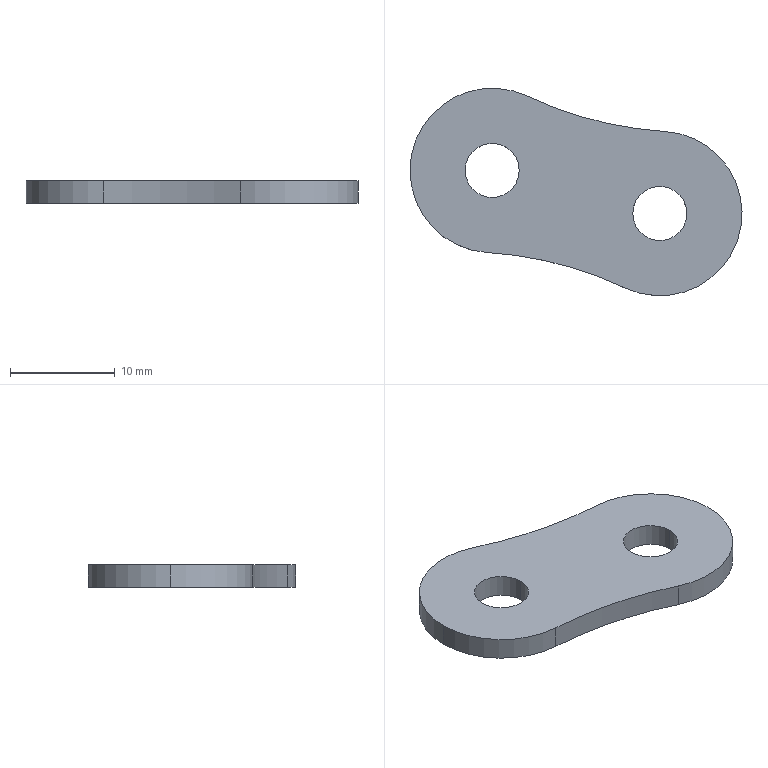Part | SolidWorks | features Boss 2, DeleteBody 1, Extrusion 1, Scale 1 | 1 solid | 11 faces | box 31.676 x 19.79 x 2.171 mm | volume 856.64 mm3 | cylinder 9 | plane 2 | commonest cylinder face diameters 5.161 x4 15.684 x2 71.994 x2 15.685 x1
STEP:
#1=CARTESIAN_POINT('',(21.666,-4.106,9.519));
#2=VERTEX_POINT('',#1);
#3=CARTESIAN_POINT('',(26.827,-4.106,9.519));
#4=VERTEX_POINT('',#3);
#5=CARTESIAN_POINT('',(24.246,-4.106,9.519));
#6=DIRECTION('',(0.,0.,1.));
#7=DIRECTION('',(1.,0.,0.));
#8=AXIS2_PLACEMENT_3D('',#5,#6,#7);
#9=CIRCLE('',#8,2.581);
#10=EDGE_CURVE('',#2,#4,#9,.T.);
#11=ORIENTED_EDGE('',*,*,#10,.T.);
#12=CARTESIAN_POINT('',(26.827,-4.106,7.348));
#13=VERTEX_POINT('',#12);
#14=CARTESIAN_POINT('',(26.827,-4.106,9.519));
#15=DIRECTION('',(0.,0.,-1.));
#16=VECTOR('',#15,1000.);
#17=LINE('',#14,#16);
#18=EDGE_CURVE('',#4,#13,#17,.T.);
#19=ORIENTED_EDGE('',*,*,#18,.T.);
#20=CARTESIAN_POINT('',(21.666,-4.106,7.348));
#21=VERTEX_POINT('',#20);
#22=CARTESIAN_POINT('',(24.246,-4.106,7.348));
#23=DIRECTION('',(0.,0.,1.));
#24=DIRECTION('',(1.,0.,0.));
#25=AXIS2_PLACEMENT_3D('',#22,#23,#24);
#26=CIRCLE('',#25,2.581);
#27=EDGE_CURVE('',#21,#13,#26,.T.);
#28=ORIENTED_EDGE('',*,*,#27,.F.);
#29=CARTESIAN_POINT('',(21.666,-4.106,9.519));
#30=DIRECTION('',(0.,0.,-1.));
#31=VECTOR('',#30,1000.);
#32=LINE('',#29,#31);
#33=EDGE_CURVE('',#2,#21,#32,.T.);
#34=ORIENTED_EDGE('',*,*,#33,.F.);
#35=EDGE_LOOP('',(#11,#19,#28,#34));
#36=FACE_OUTER_BOUND('',#35,.T.);
#37=CARTESIAN_POINT('',(24.246,-4.106,9.519));
#38=DIRECTION('',(0.,0.,-1.));
#39=DIRECTION('',(-1.,0.,0.));
#40=AXIS2_PLACEMENT_3D('',#37,#38,#39);
#41=CYLINDRICAL_SURFACE('',#40,2.581);
#42=ADVANCED_FACE('',(#36),#41,.F.);
#43=CARTESIAN_POINT('',(5.675,0.,9.519));
#44=VERTEX_POINT('',#43);
#45=CARTESIAN_POINT('',(10.836,0.,9.519));
#46=VERTEX_POINT('',#45);
#47=CARTESIAN_POINT('',(8.255,0.,9.519));
#48=DIRECTION('',(0.,0.,1.));
#49=DIRECTION('',(1.,0.,0.));
#50=AXIS2_PLACEMENT_3D('',#47,#48,#49);
#51=CIRCLE('',#50,2.58);
#52=EDGE_CURVE('',#44,#46,#51,.T.);
#53=ORIENTED_EDGE('',*,*,#52,.T.);
#54=CARTESIAN_POINT('',(10.836,0.,7.348));
#55=VERTEX_POINT('',#54);
#56=CARTESIAN_POINT('',(10.836,0.,9.519));
#57=DIRECTION('',(0.,0.,-1.));
#58=VECTOR('',#57,1000.);
#59=LINE('',#56,#58);
#60=EDGE_CURVE('',#46,#55,#59,.T.);
#61=ORIENTED_EDGE('',*,*,#60,.T.);
#62=CARTESIAN_POINT('',(5.675,0.,7.348));
#63=VERTEX_POINT('',#62);
#64=CARTESIAN_POINT('',(8.255,0.,7.348));
#65=DIRECTION('',(0.,0.,1.));
#66=DIRECTION('',(1.,0.,0.));
#67=AXIS2_PLACEMENT_3D('',#64,#65,#66);
#68=CIRCLE('',#67,2.58);
#69=EDGE_CURVE('',#63,#55,#68,.T.);
#70=ORIENTED_EDGE('',*,*,#69,.F.);
#71=CARTESIAN_POINT('',(5.675,0.,9.519));
#72=DIRECTION('',(0.,0.,-1.));
#73=VECTOR('',#72,1000.);
#74=LINE('',#71,#73);
#75=EDGE_CURVE('',#44,#63,#74,.T.);
#76=ORIENTED_EDGE('',*,*,#75,.F.);
#77=EDGE_LOOP('',(#53,#61,#70,#76));
#78=FACE_OUTER_BOUND('',#77,.T.);
#79=CARTESIAN_POINT('',(8.255,0.,9.519));
#80=DIRECTION('',(0.,0.,-1.));
#81=DIRECTION('',(-1.,0.,0.));
#82=AXIS2_PLACEMENT_3D('',#79,#80,#81);
#83=CYLINDRICAL_SURFACE('',#82,2.581);
#84=ADVANCED_FACE('',(#78),#83,.F.);
#85=CARTESIAN_POINT('',(0.4128,0.,9.519));
#86=VERTEX_POINT('',#85);
#87=CARTESIAN_POINT('',(7.77,-7.827,9.519));
#88=VERTEX_POINT('',#87);
#89=CARTESIAN_POINT('',(8.255,0.,9.519));
#90=DIRECTION('',(0.,0.,1.));
#91=DIRECTION('',(1.,0.,0.));
#92=AXIS2_PLACEMENT_3D('',#89,#90,#91);
#93=CIRCLE('',#92,7.842);
#94=EDGE_CURVE('',#86,#88,#93,.T.);
#95=ORIENTED_EDGE('',*,*,#94,.F.);
#96=CARTESIAN_POINT('',(0.4128,0.,7.348));
#97=VERTEX_POINT('',#96);
#98=CARTESIAN_POINT('',(0.4128,0.,9.519));
#99=DIRECTION('',(0.,0.,-1.));
#100=VECTOR('',#99,1000.);
#101=LINE('',#98,#100);
#102=EDGE_CURVE('',#86,#97,#101,.T.);
#103=ORIENTED_EDGE('',*,*,#102,.T.);
#104=CARTESIAN_POINT('',(7.77,-7.827,7.348));
#105=VERTEX_POINT('',#104);
#106=CARTESIAN_POINT('',(8.255,0.,7.348));
#107=DIRECTION('',(0.,0.,1.));
#108=DIRECTION('',(1.,0.,0.));
#109=AXIS2_PLACEMENT_3D('',#106,#107,#108);
#110=CIRCLE('',#109,7.842);
#111=EDGE_CURVE('',#97,#105,#110,.T.);
#112=ORIENTED_EDGE('',*,*,#111,.T.);
#113=CARTESIAN_POINT('',(7.77,-7.827,9.519));
#114=DIRECTION('',(0.,0.,-1.));
#115=VECTOR('',#114,1000.);
#116=LINE('',#113,#115);
#117=EDGE_CURVE('',#88,#105,#116,.T.);
#118=ORIENTED_EDGE('',*,*,#117,.F.);
#119=EDGE_LOOP('',(#95,#103,#112,#118));
#120=FACE_OUTER_BOUND('',#119,.T.);
#121=CARTESIAN_POINT('',(8.255,0.,9.519));
#122=DIRECTION('',(0.,0.,-1.));
#123=DIRECTION('',(-1.,0.,0.));
#124=AXIS2_PLACEMENT_3D('',#121,#122,#123);
#125=CYLINDRICAL_SURFACE('',#124,7.842);
#126=ADVANCED_FACE('',(#120),#125,.T.);
#127=ORIENTED_EDGE('',*,*,#52,.F.);
#128=CARTESIAN_POINT('',(8.255,0.,9.519));
#129=DIRECTION('',(0.,0.,1.));
#130=DIRECTION('',(1.,0.,0.));
#131=AXIS2_PLACEMENT_3D('',#128,#129,#130);
#132=CIRCLE('',#131,2.58);
#133=EDGE_CURVE('',#46,#44,#132,.T.);
#134=ORIENTED_EDGE('',*,*,#133,.F.);
#135=EDGE_LOOP('',(#127,#134));
#136=FACE_BOUND('',#135,.T.);
#137=CARTESIAN_POINT('',(24.731,3.721,9.519));
#138=VERTEX_POINT('',#137);
#139=CARTESIAN_POINT('',(11.601,7.093,9.519));
#140=VERTEX_POINT('',#139);
#141=CARTESIAN_POINT('',(26.958,39.65,9.519));
#142=DIRECTION('',(0.,0.,-1.));
#143=DIRECTION('',(1.,0.,0.));
#144=AXIS2_PLACEMENT_3D('',#141,#142,#143);
#145=CIRCLE('',#144,35.997);
#146=EDGE_CURVE('',#138,#140,#145,.T.);
#147=ORIENTED_EDGE('',*,*,#146,.T.);
#148=CARTESIAN_POINT('',(8.255,0.,9.519));
#149=DIRECTION('',(0.,0.,1.));
#150=DIRECTION('',(1.,0.,0.));
#151=AXIS2_PLACEMENT_3D('',#148,#149,#150);
#152=CIRCLE('',#151,7.842);
#153=EDGE_CURVE('',#140,#86,#152,.T.);
#154=ORIENTED_EDGE('',*,*,#153,.T.);
#155=ORIENTED_EDGE('',*,*,#94,.T.);
#156=CARTESIAN_POINT('',(20.901,-11.199,9.519));
#157=VERTEX_POINT('',#156);
#158=CARTESIAN_POINT('',(5.543,-43.756,9.519));
#159=DIRECTION('',(0.,0.,-1.));
#160=DIRECTION('',(-1.,0.,0.));
#161=AXIS2_PLACEMENT_3D('',#158,#159,#160);
#162=CIRCLE('',#161,35.997);
#163=EDGE_CURVE('',#88,#157,#162,.T.);
#164=ORIENTED_EDGE('',*,*,#163,.T.);
#165=CARTESIAN_POINT('',(24.246,-4.106,9.519));
#166=DIRECTION('',(0.,0.,1.));
#167=DIRECTION('',(1.,0.,0.));
#168=AXIS2_PLACEMENT_3D('',#165,#166,#167);
#169=CIRCLE('',#168,7.842);
#170=EDGE_CURVE('',#157,#138,#169,.T.);
#171=ORIENTED_EDGE('',*,*,#170,.T.);
#172=EDGE_LOOP('',(#147,#154,#155,#164,#171));
#173=FACE_OUTER_BOUND('',#172,.T.);
#174=ORIENTED_EDGE('',*,*,#10,.F.);
#175=CARTESIAN_POINT('',(24.246,-4.106,9.519));
#176=DIRECTION('',(0.,0.,1.));
#177=DIRECTION('',(1.,0.,0.));
#178=AXIS2_PLACEMENT_3D('',#175,#176,#177);
#179=CIRCLE('',#178,2.581);
#180=EDGE_CURVE('',#4,#2,#179,.T.);
#181=ORIENTED_EDGE('',*,*,#180,.F.);
#182=EDGE_LOOP('',(#174,#181));
#183=FACE_BOUND('',#182,.T.);
#184=CARTESIAN_POINT('',(25.602,17.772,9.519));
#185=DIRECTION('',(0.,0.,1.));
#186=DIRECTION('',(1.,0.,0.));
#187=AXIS2_PLACEMENT_3D('',#184,#185,#186);
#188=PLANE('',#187);
#189=ADVANCED_FACE('',(#136,#173,#183),#188,.T.);
#190=ORIENTED_EDGE('',*,*,#69,.T.);
#191=CARTESIAN_POINT('',(8.255,0.,7.348));
#192=DIRECTION('',(0.,0.,1.));
#193=DIRECTION('',(1.,0.,0.));
#194=AXIS2_PLACEMENT_3D('',#191,#192,#193);
#195=CIRCLE('',#194,2.58);
#196=EDGE_CURVE('',#55,#63,#195,.T.);
#197=ORIENTED_EDGE('',*,*,#196,.T.);
#198=EDGE_LOOP('',(#190,#197));
#199=FACE_BOUND('',#198,.T.);
#200=CARTESIAN_POINT('',(24.731,3.721,7.348));
#201=VERTEX_POINT('',#200);
#202=CARTESIAN_POINT('',(11.601,7.093,7.348));
#203=VERTEX_POINT('',#202);
#204=CARTESIAN_POINT('',(26.958,39.65,7.348));
#205=DIRECTION('',(0.,0.,-1.));
#206=DIRECTION('',(1.,0.,0.));
#207=AXIS2_PLACEMENT_3D('',#204,#205,#206);
#208=CIRCLE('',#207,35.997);
#209=EDGE_CURVE('',#201,#203,#208,.T.);
#210=ORIENTED_EDGE('',*,*,#209,.F.);
#211=CARTESIAN_POINT('',(20.901,-11.199,7.348));
#212=VERTEX_POINT('',#211);
#213=CARTESIAN_POINT('',(24.246,-4.106,7.348));
#214=DIRECTION('',(0.,0.,1.));
#215=DIRECTION('',(1.,0.,0.));
#216=AXIS2_PLACEMENT_3D('',#213,#214,#215);
#217=CIRCLE('',#216,7.842);
#218=EDGE_CURVE('',#212,#201,#217,.T.);
#219=ORIENTED_EDGE('',*,*,#218,.F.);
#220=CARTESIAN_POINT('',(5.543,-43.756,7.348));
#221=DIRECTION('',(0.,0.,-1.));
#222=DIRECTION('',(-1.,0.,0.));
#223=AXIS2_PLACEMENT_3D('',#220,#221,#222);
#224=CIRCLE('',#223,35.997);
#225=EDGE_CURVE('',#105,#212,#224,.T.);
#226=ORIENTED_EDGE('',*,*,#225,.F.);
#227=ORIENTED_EDGE('',*,*,#111,.F.);
#228=CARTESIAN_POINT('',(8.255,0.,7.348));
#229=DIRECTION('',(0.,0.,1.));
#230=DIRECTION('',(1.,0.,0.));
#231=AXIS2_PLACEMENT_3D('',#228,#229,#230);
#232=CIRCLE('',#231,7.842);
#233=EDGE_CURVE('',#203,#97,#232,.T.);
#234=ORIENTED_EDGE('',*,*,#233,.F.);
#235=EDGE_LOOP('',(#210,#219,#226,#227,#234));
#236=FACE_OUTER_BOUND('',#235,.T.);
#237=ORIENTED_EDGE('',*,*,#27,.T.);
#238=CARTESIAN_POINT('',(24.246,-4.106,7.348));
#239=DIRECTION('',(0.,0.,1.));
#240=DIRECTION('',(1.,0.,0.));
#241=AXIS2_PLACEMENT_3D('',#238,#239,#240);
#242=CIRCLE('',#241,2.581);
#243=EDGE_CURVE('',#13,#21,#242,.T.);
#244=ORIENTED_EDGE('',*,*,#243,.T.);
#245=EDGE_LOOP('',(#237,#244));
#246=FACE_BOUND('',#245,.T.);
#247=CARTESIAN_POINT('',(25.602,17.772,7.348));
#248=DIRECTION('',(0.,0.,1.));
#249=DIRECTION('',(1.,0.,0.));
#250=AXIS2_PLACEMENT_3D('',#247,#248,#249);
#251=PLANE('',#250);
#252=ADVANCED_FACE('',(#199,#236,#246),#251,.F.);
#253=ORIENTED_EDGE('',*,*,#209,.T.);
#254=CARTESIAN_POINT('',(11.601,7.093,9.519));
#255=DIRECTION('',(0.,0.,-1.));
#256=VECTOR('',#255,1000.);
#257=LINE('',#254,#256);
#258=EDGE_CURVE('',#140,#203,#257,.T.);
#259=ORIENTED_EDGE('',*,*,#258,.F.);
#260=ORIENTED_EDGE('',*,*,#146,.F.);
#261=CARTESIAN_POINT('',(24.731,3.721,9.519));
#262=DIRECTION('',(0.,0.,-1.));
#263=VECTOR('',#262,1000.);
#264=LINE('',#261,#263);
#265=EDGE_CURVE('',#138,#201,#264,.T.);
#266=ORIENTED_EDGE('',*,*,#265,.T.);
#267=EDGE_LOOP('',(#253,#259,#260,#266));
#268=FACE_OUTER_BOUND('',#267,.T.);
#269=CARTESIAN_POINT('',(26.958,39.65,9.519));
#270=DIRECTION('',(0.,0.,-1.));
#271=DIRECTION('',(-1.,0.,0.));
#272=AXIS2_PLACEMENT_3D('',#269,#270,#271);
#273=CYLINDRICAL_SURFACE('',#272,35.997);
#274=ADVANCED_FACE('',(#268),#273,.F.);
#275=ORIENTED_EDGE('',*,*,#102,.F.);
#276=ORIENTED_EDGE('',*,*,#153,.F.);
#277=ORIENTED_EDGE('',*,*,#258,.T.);
#278=ORIENTED_EDGE('',*,*,#233,.T.);
#279=EDGE_LOOP('',(#275,#276,#277,#278));
#280=FACE_OUTER_BOUND('',#279,.T.);
#281=CARTESIAN_POINT('',(8.255,0.,9.519));
#282=DIRECTION('',(0.,0.,-1.));
#283=DIRECTION('',(-1.,0.,0.));
#284=AXIS2_PLACEMENT_3D('',#281,#282,#283);
#285=CYLINDRICAL_SURFACE('',#284,7.842);
#286=ADVANCED_FACE('',(#280),#285,.T.);
#287=ORIENTED_EDGE('',*,*,#225,.T.);
#288=CARTESIAN_POINT('',(20.901,-11.199,9.519));
#289=DIRECTION('',(0.,0.,-1.));
#290=VECTOR('',#289,1000.);
#291=LINE('',#288,#290);
#292=EDGE_CURVE('',#157,#212,#291,.T.);
#293=ORIENTED_EDGE('',*,*,#292,.F.);
#294=ORIENTED_EDGE('',*,*,#163,.F.);
#295=ORIENTED_EDGE('',*,*,#117,.T.);
#296=EDGE_LOOP('',(#287,#293,#294,#295));
#297=FACE_OUTER_BOUND('',#296,.T.);
#298=CARTESIAN_POINT('',(5.543,-43.756,9.519));
#299=DIRECTION('',(0.,0.,-1.));
#300=DIRECTION('',(-1.,0.,0.));
#301=AXIS2_PLACEMENT_3D('',#298,#299,#300);
#302=CYLINDRICAL_SURFACE('',#301,35.997);
#303=ADVANCED_FACE('',(#297),#302,.F.);
#304=ORIENTED_EDGE('',*,*,#218,.T.);
#305=ORIENTED_EDGE('',*,*,#265,.F.);
#306=ORIENTED_EDGE('',*,*,#170,.F.);
#307=ORIENTED_EDGE('',*,*,#292,.T.);
#308=EDGE_LOOP('',(#304,#305,#306,#307));
#309=FACE_OUTER_BOUND('',#308,.T.);
#310=CARTESIAN_POINT('',(24.246,-4.106,9.519));
#311=DIRECTION('',(0.,0.,-1.));
#312=DIRECTION('',(-1.,0.,0.));
#313=AXIS2_PLACEMENT_3D('',#310,#311,#312);
#314=CYLINDRICAL_SURFACE('',#313,7.842);
#315=ADVANCED_FACE('',(#309),#314,.T.);
#316=ORIENTED_EDGE('',*,*,#60,.F.);
#317=ORIENTED_EDGE('',*,*,#133,.T.);
#318=ORIENTED_EDGE('',*,*,#75,.T.);
#319=ORIENTED_EDGE('',*,*,#196,.F.);
#320=EDGE_LOOP('',(#316,#317,#318,#319));
#321=FACE_OUTER_BOUND('',#320,.T.);
#322=CARTESIAN_POINT('',(8.255,0.,9.519));
#323=DIRECTION('',(0.,0.,-1.));
#324=DIRECTION('',(-1.,0.,0.));
#325=AXIS2_PLACEMENT_3D('',#322,#323,#324);
#326=CYLINDRICAL_SURFACE('',#325,2.581);
#327=ADVANCED_FACE('',(#321),#326,.F.);
#328=ORIENTED_EDGE('',*,*,#18,.F.);
#329=ORIENTED_EDGE('',*,*,#180,.T.);
#330=ORIENTED_EDGE('',*,*,#33,.T.);
#331=ORIENTED_EDGE('',*,*,#243,.F.);
#332=EDGE_LOOP('',(#328,#329,#330,#331));
#333=FACE_OUTER_BOUND('',#332,.T.);
#334=CARTESIAN_POINT('',(24.246,-4.106,9.519));
#335=DIRECTION('',(0.,0.,-1.));
#336=DIRECTION('',(-1.,0.,0.));
#337=AXIS2_PLACEMENT_3D('',#334,#335,#336);
#338=CYLINDRICAL_SURFACE('',#337,2.581);
#339=ADVANCED_FACE('',(#333),#338,.F.);
#340=CLOSED_SHELL('',(#42,#84,#126,#189,#252,#274,#286,#303,#315,#327,#339));
#341=MANIFOLD_SOLID_BREP('',#340);
#342=CARTESIAN_POINT('',(0.,0.,0.));
#343=DIRECTION('',(0.,0.,1.));
#344=DIRECTION('',(1.,0.,0.));
#345=AXIS2_PLACEMENT_3D('',#342,#343,#344);
#346=(LENGTH_UNIT()NAMED_UNIT(*)SI_UNIT(.MILLI.,.METRE.));
#347=UNCERTAINTY_MEASURE_WITH_UNIT(LENGTH_MEASURE(0.00001),#346,'','');
#348=(NAMED_UNIT(*)PLANE_ANGLE_UNIT()SI_UNIT($,.RADIAN.));
#349=(NAMED_UNIT(*)SI_UNIT($,.STERADIAN.)SOLID_ANGLE_UNIT());
#350=(GEOMETRIC_REPRESENTATION_CONTEXT(3)GLOBAL_UNCERTAINTY_ASSIGNED_CONTEXT((#347))GLOBAL_UNIT_ASSIGNED_CONTEXT((#346,#348,#349))REPRESENTATION_CONTEXT('',''));
#351=ADVANCED_BREP_SHAPE_REPRESENTATION('',(#341,#345),#350);